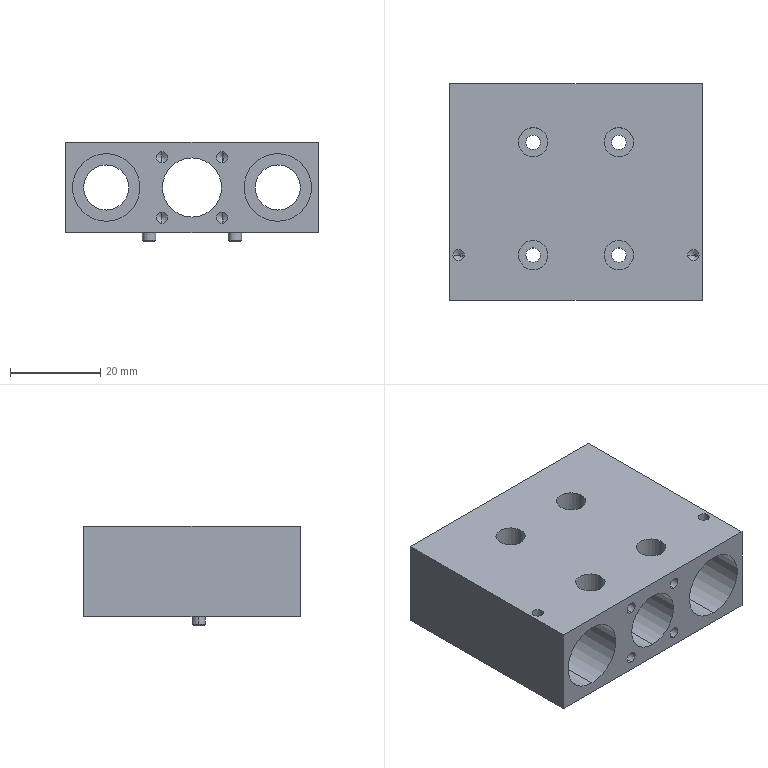Part | 1 solid | 72 faces | box 56 x 48 x 22 mm | volume 29622 mm3 | cylinder 42 | cone 16 | plane 14 | commonest cylinder face diameters 2.5 x12 3.2 x8 6.5 x8 3 x4 10 x4 15 x4